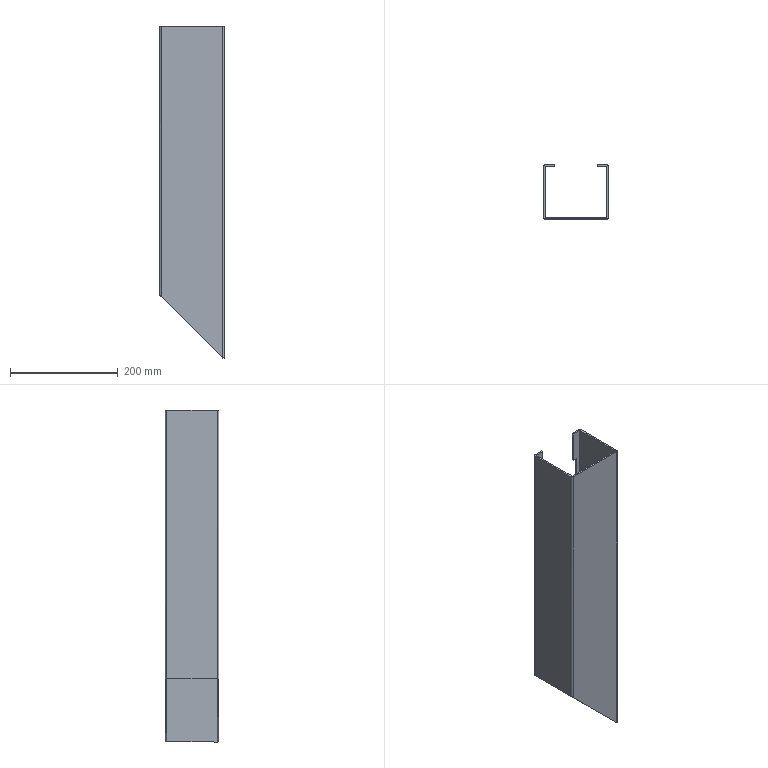Part | STEP file | TS-008-01 | 1 solid | 54 faces | box 120 x 100 x 615 mm | volume 571993 mm3 | plane 42 | cylinder 8 | spline 4 | commonest cylinder face diameters 0.4 x4 6.4 x4